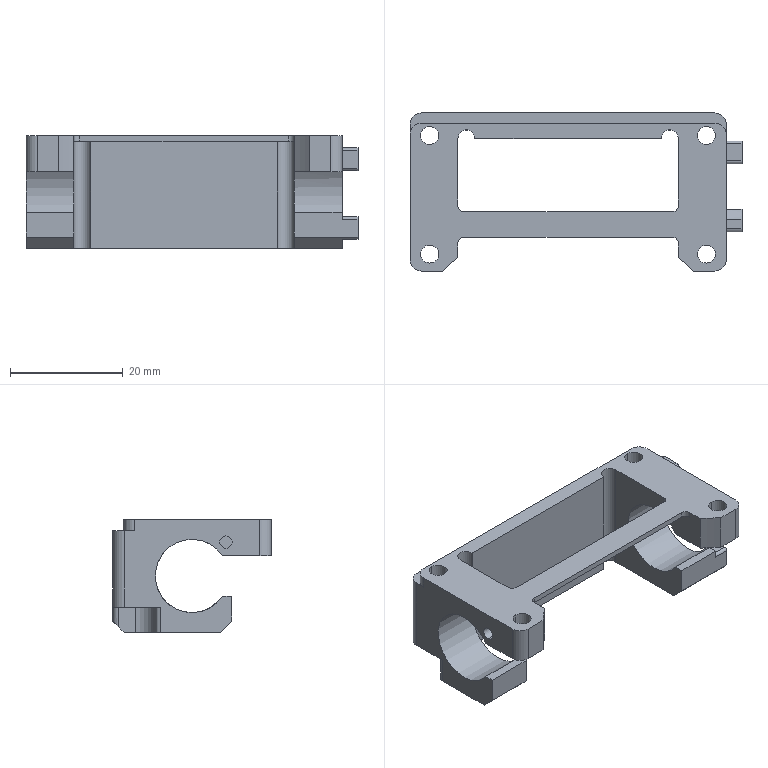NC program | Mastercam | posted with a generic post | part box 58.8 x 28 x 20 mm
Lines 3433 to 4298 of 29451:
(6 FEM |TOOL - 6|DIA. OFF. - 6|LEN. - 6|TOOL DIA. - 6.)
N6930 T6 M6
N6932 G0 G54 G90 X27.5 Y13.92 C0. B0. S6500 M3
N6934 G43 H6 Z50.
N6936 Z.11
N6938 G1 X27.215 Y13.9 Z.1 F2500.
N6940 X26.937 Y13.839 Z.09
N6942 X26.669 Y13.739 Z.08
N6944 X26.419 Y13.603 Z.07
N6946 X26.19 Y13.432 Z.06
N6948 X25.989 Y13.23 Z.05
N6950 X25.817 Y13.001 Z.04
N6952 X25.681 Y12.751 Z.03
N6954 X25.581 Y12.484 Z.02
N6956 X25.52 Y12.205 Z.01
N6958 X25.5 Y11.92 Z0.
N6960 Y10.158
N6962 X25.523 Y9.924
N6964 X25.581 Y9.785
N6966 X25.686 Y9.68
N6968 X25.825 Y9.622
N6970 X27.799 Y9.6
N6972 X28.084 Y9.617 Z.01
N6974 X28.364 Y9.675 Z.02
N6976 X28.632 Y9.771 Z.03
N6978 X28.884 Y9.905 Z.04
N6980 X29.115 Y10.074 Z.05
N6982 X29.319 Y10.273 Z.06
N6984 X29.492 Y10.5 Z.07
N6986 X29.632 Y10.748 Z.08
N6988 X29.735 Y11.015 Z.09
N6990 X29.798 Y11.293 Z.1
N6992 X29.822 Y11.577 Z.11
N6994 X29.823 Y11.655
N6996 X29.825 Y11.731 Z.109
N6998 X29.826 Y11.805
N7000 X29.828 Y11.878 Z.108
N7002 X29.831 Y11.95 Z.107
N7004 X29.833 Y12.02
N7006 X29.836 Y12.088 Z.105
N7008 X29.839 Y12.155 Z.104
N7010 X29.846 Y12.285 Z.101
N7012 X29.853 Y12.408 Z.097
N7014 X29.862 Y12.526 Z.093
N7016 X29.87 Y12.639 Z.088
N7018 X29.88 Y12.746 Z.083
N7020 X29.889 Y12.848 Z.077
N7022 X29.899 Y12.945 Z.07
N7024 X29.909 Y13.037 Z.064
N7026 X29.918 Y13.124 Z.056
N7028 X29.928 Y13.206 Z.048
N7030 X29.937 Y13.284 Z.04
N7032 X29.946 Y13.357 Z.032
N7034 X29.954 Y13.426 Z.023
N7036 X29.962 Y13.49 Z.013
N7038 X29.974 Y13.606 Z-.006
N7040 X29.983 Y13.707 Z-.027
N7042 X29.985 Y13.752 Z-.038
N7044 X29.986 Y13.793 Z-.048
N7046 Y13.831 Z-.06
N7048 X29.984 Y13.865 Z-.071
N7050 X29.98 Y13.897 Z-.082
N7052 X29.974 Y13.925 Z-.094
N7054 X29.966 Y13.95 Z-.105
N7056 X29.956 Y13.973 Z-.117
N7058 X29.944 Y13.993 Z-.129
N7060 X29.93 Y14.01 Z-.14
N7062 X29.913 Y14.025 Z-.152
N7064 X29.894 Y14.037 Z-.164
N7066 X29.871 Y14.048 Z-.175
N7068 X29.846 Y14.056 Z-.187
N7070 X29.818 Y14.062 Z-.198
N7072 X29.787 Y14.067 Z-.21
N7074 X29.753 Y14.069 Z-.221
N7076 X29.715 Y14.07 Z-.232
N7078 X29.674 Z-.243
N7080 X29.629 Y14.068 Z-.254
N7082 X29.529 Y14.061 Z-.274
N7084 X29.413 Y14.05 Z-.294
N7086 X29.348 Y14.043 Z-.303
N7088 X29.28 Y14.036 Z-.312
N7090 X29.207 Y14.028 Z-.321
N7092 X29.129 Y14.02 Z-.329
N7094 X29.047 Y14.012 Z-.337
N7096 X28.96 Y14.003 Z-.344
N7098 X28.868 Y13.994 Z-.351
N7100 X28.771 Y13.986 Z-.357
N7102 X28.669 Y13.978 Z-.363
N7104 X28.562 Y13.97 Z-.369
N7106 X28.449 Y13.962 Z-.374
N7108 X28.331 Y13.955 Z-.378
N7110 X28.207 Y13.949 Z-.382
N7112 X28.078 Y13.944 Z-.385
N7114 X28.011 Y13.942 Z-.386
N7116 X27.942 Y13.94 Z-.387
N7118 X27.873 Y13.938 Z-.388
N7120 X27.801 Y13.936 Z-.389
N7122 X27.728 Y13.935
N7124 X27.654 Y13.934 Z-.39
N7126 X27.578
N7128 X27.5
N7130 X27.215 Y13.913 Z-.4
N7132 X26.936 Y13.853 Z-.41
N7134 X26.669 Y13.753 Z-.42
N7136 X26.419 Y13.616 Z-.43
N7138 X26.19 Y13.445 Z-.44
N7140 X25.988 Y13.243 Z-.45
N7142 X25.817 Y13.015 Z-.46
N7144 X25.681 Y12.765 Z-.47
N7146 X25.581 Y12.497 Z-.48
N7148 X25.52 Y12.218 Z-.49
N7150 X25.5 Y11.934 Z-.5
N7152 Y10.158
N7154 X25.523 Y9.924
N7156 X25.581 Y9.785
N7158 X25.686 Y9.68
N7160 X25.825 Y9.622
N7162 X27.799 Y9.6
N7164 X28.084 Y9.617 Z-.49
N7166 X28.364 Y9.675 Z-.48
N7168 X28.632 Y9.771 Z-.47
N7170 X28.884 Y9.905 Z-.46
N7172 X29.115 Y10.074 Z-.45
N7174 X29.319 Y10.273 Z-.44
N7176 X29.492 Y10.5 Z-.43
N7178 X29.632 Y10.748 Z-.42
N7180 X29.735 Y11.015 Z-.41
N7182 X29.798 Y11.293 Z-.4
N7184 X29.822 Y11.577 Z-.39
N7186 X29.823 Y11.655
N7188 X29.824 Y11.73 Z-.391
N7190 X29.826 Y11.805
N7192 X29.828 Y11.877 Z-.392
N7194 X29.83 Y11.949 Z-.393
N7196 X29.833 Y12.018
N7198 X29.836 Y12.087 Z-.395
N7200 X29.839 Y12.153 Z-.396
N7202 X29.846 Y12.282 Z-.399
N7204 X29.853 Y12.406 Z-.403
N7206 X29.861 Y12.523 Z-.407
N7208 X29.87 Y12.636 Z-.412
N7210 X29.879 Y12.743 Z-.417
N7212 X29.889 Y12.844 Z-.423
N7214 X29.898 Y12.941 Z-.43
N7216 X29.908 Y13.032 Z-.436
N7218 X29.917 Y13.119 Z-.444
N7220 X29.927 Y13.201 Z-.452
N7222 X29.936 Y13.278 Z-.46
N7224 X29.944 Y13.351 Z-.468
N7226 X29.952 Y13.419 Z-.477
N7228 X29.96 Y13.483 Z-.487
N7230 X29.972 Y13.599 Z-.506
N7232 X29.98 Y13.699 Z-.527
N7234 X29.983 Y13.744 Z-.538
N7236 X29.984 Y13.785 Z-.548
N7238 X29.983 Y13.822 Z-.56
N7240 X29.981 Y13.856 Z-.571
N7242 X29.977 Y13.888 Z-.582
N7244 X29.971 Y13.916 Z-.594
N7246 X29.963 Y13.941 Z-.605
N7248 X29.953 Y13.963 Z-.617
N7250 X29.941 Y13.983 Z-.629
N7252 X29.926 Y14. Z-.64
N7254 X29.909 Y14.014 Z-.652
N7256 X29.89 Y14.027 Z-.664
N7258 X29.867 Y14.037 Z-.675
N7260 X29.842 Y14.045 Z-.687
N7262 X29.814 Y14.051 Z-.698
N7264 X29.783 Y14.055 Z-.71
N7266 X29.749 Y14.057 Z-.721
N7268 X29.711 Y14.058 Z-.732
N7270 X29.67 Z-.743
N7272 X29.625 Y14.056 Z-.754
N7274 X29.525 Y14.049 Z-.774
N7276 X29.408 Y14.037 Z-.794
N7278 X29.344 Y14.031 Z-.803
N7280 X29.276 Y14.023 Z-.812
N7282 X29.203 Y14.015 Z-.821
N7284 X29.125 Y14.007 Z-.829
N7286 X29.043 Y13.998 Z-.837
N7288 X28.956 Y13.99 Z-.844
N7290 X28.865 Y13.981 Z-.851
N7292 X28.768 Y13.973 Z-.857
N7294 X28.666 Y13.964 Z-.863
N7296 X28.559 Y13.956 Z-.869
N7298 X28.447 Y13.949 Z-.874
N7300 X28.329 Y13.942 Z-.878
N7302 X28.205 Y13.936 Z-.882
N7304 X28.076 Y13.93 Z-.885
N7306 X28.01 Y13.928 Z-.886
N7308 X27.941 Y13.926 Z-.887
N7310 X27.872 Y13.924 Z-.888
N7312 X27.8 Y13.923 Z-.889
N7314 X27.728 Y13.922
N7316 X27.653 Y13.921 Z-.89
N7318 X27.577 Y13.92
N7320 X27.5
N7322 X27.215 Y13.9 Z-.9
N7324 X26.937 Y13.839 Z-.91
N7326 X26.669 Y13.739 Z-.92
N7328 X26.419 Y13.603 Z-.93
N7330 X26.19 Y13.432 Z-.94
N7332 X25.989 Y13.23 Z-.95
N7334 X25.817 Y13.001 Z-.96
N7336 X25.681 Y12.751 Z-.97
N7338 X25.581 Y12.484 Z-.98
N7340 X25.52 Y12.205 Z-.99
N7342 X25.5 Y11.92 Z-1.
N7344 Y10.158
N7346 X25.523 Y9.924
N7348 X25.581 Y9.785
N7350 X25.686 Y9.68
N7352 X25.825 Y9.622
N7354 X27.799 Y9.6
N7356 X28.084 Y9.617 Z-.99
N7358 X28.364 Y9.675 Z-.98
N7360 X28.632 Y9.771 Z-.97
N7362 X28.884 Y9.905 Z-.96
N7364 X29.115 Y10.074 Z-.95
N7366 X29.319 Y10.273 Z-.94
N7368 X29.492 Y10.5 Z-.93
N7370 X29.632 Y10.748 Z-.92
N7372 X29.735 Y11.015 Z-.91
N7374 X29.798 Y11.293 Z-.9
N7376 X29.822 Y11.577 Z-.89
N7378 X29.823 Y11.655
N7380 X29.824 Y11.73 Z-.891
N7382 X29.826 Y11.805
N7384 X29.828 Y11.877 Z-.892
N7386 X29.83 Y11.949 Z-.893
N7388 X29.833 Y12.018
N7390 X29.836 Y12.086 Z-.895
N7392 X29.839 Y12.153 Z-.896
N7394 X29.846 Y12.282 Z-.899
N7396 X29.853 Y12.406 Z-.903
N7398 X29.861 Y12.523 Z-.907
N7400 X29.87 Y12.635 Z-.912
N7402 X29.879 Y12.742 Z-.917
N7404 X29.888 Y12.844 Z-.923
N7406 X29.898 Y12.94 Z-.929
N7408 X29.908 Y13.032 Z-.936
N7410 X29.917 Y13.119 Z-.943
N7412 X29.927 Y13.2 Z-.951
N7414 X29.936 Y13.278 Z-.959
N7416 X29.944 Y13.35 Z-.968
N7418 X29.952 Y13.419 Z-.977
N7420 X29.96 Y13.483 Z-.986
N7422 X29.972 Y13.599 Z-1.005
N7424 X29.98 Y13.699 Z-1.026
N7426 X29.983 Y13.743 Z-1.036
N7428 Y13.784 Z-1.047
N7430 Y13.822 Z-1.058
N7432 X29.981 Y13.856 Z-1.069
N7434 X29.977 Y13.887 Z-1.08
N7436 X29.971 Y13.915 Z-1.092
N7438 X29.963 Y13.94 Z-1.103
N7440 X29.953 Y13.963 Z-1.115
N7442 X29.941 Y13.982 Z-1.126
N7444 X29.926 Y13.999 Z-1.138
N7446 X29.909 Y14.014 Z-1.15
N7448 X29.889 Y14.026 Z-1.161
N7450 X29.867 Y14.036 Z-1.173
N7452 X29.842 Y14.044 Z-1.184
N7454 X29.814 Y14.051 Z-1.195
N7456 X29.783 Y14.055 Z-1.207
N7458 X29.748 Y14.057 Z-1.218
N7460 X29.711 Y14.058 Z-1.229
N7462 X29.669 Z-1.24
N7464 X29.625 Y14.056 Z-1.25
N7466 X29.524 Y14.048 Z-1.271
N7468 X29.408 Y14.037 Z-1.29
N7470 X29.344 Y14.03 Z-1.299
N7472 X29.275 Y14.023 Z-1.308
N7474 X29.202 Y14.015 Z-1.317
N7476 X29.125 Y14.007 Z-1.325
N7478 X29.043 Y13.998 Z-1.333
N7480 X28.956 Y13.99 Z-1.34
N7482 X28.864 Y13.981 Z-1.347
N7484 X28.768 Y13.972 Z-1.353
N7486 X28.666 Y13.964 Z-1.359
N7488 X28.559 Y13.956 Z-1.364
N7490 X28.447 Y13.949 Z-1.369
N7492 X28.329 Y13.942 Z-1.373
N7494 X28.205 Y13.936 Z-1.377
N7496 X28.076 Y13.93 Z-1.38
N7498 X28.009 Y13.928 Z-1.381
N7500 X27.941 Y13.926 Z-1.382
N7502 X27.871 Y13.924 Z-1.383
N7504 X27.8 Y13.923 Z-1.384
N7506 X27.727 Y13.922 Z-1.385
N7508 X27.653 Y13.921
N7510 X27.577 Y13.92
N7512 X27.5 Z-1.386
N7514 X27.215 Y13.9 Z-1.396
N7516 X26.937 Y13.839 Z-1.406
N7518 X26.669 Y13.739 Z-1.415
N7520 X26.419 Y13.603 Z-1.425
N7522 X26.19 Y13.432 Z-1.435
N7524 X25.989 Y13.23 Z-1.445
N7526 X25.817 Y13.001 Z-1.455
N7528 X25.681 Y12.751 Z-1.465
N7530 X25.581 Y12.484 Z-1.475
N7532 X25.52 Y12.205 Z-1.485
N7534 X25.5 Y11.92 Z-1.495
N7536 Y10.158
N7538 X25.523 Y9.924
N7540 X25.581 Y9.785
N7542 X25.686 Y9.68
N7544 X25.825 Y9.622
N7546 X27.799 Y9.6
N7548 X28.084 Y9.617 Z-1.485
N7550 X28.364 Y9.675 Z-1.475
N7552 X28.632 Y9.771 Z-1.465
N7554 X28.884 Y9.905 Z-1.455
N7556 X29.115 Y10.074 Z-1.445
N7558 X29.319 Y10.273 Z-1.435
N7560 X29.492 Y10.5 Z-1.425
N7562 X29.632 Y10.748 Z-1.415
N7564 X29.735 Y11.015 Z-1.406
N7566 X29.798 Y11.293 Z-1.396
N7568 X29.822 Y11.577 Z-1.386
N7570 X29.823 Y11.654
N7572 X29.824 Y11.729
N7574 X29.826 Y11.803
N7576 X29.828 Y11.875
N7578 X29.83 Y11.946 Z-1.387
N7580 X29.833 Y12.015
N7582 X29.836 Y12.082 Z-1.388
N7584 X29.838 Y12.149
N7586 X29.845 Y12.277 Z-1.39
N7588 X29.852 Y12.399 Z-1.392
N7590 X29.86 Y12.516 Z-1.394
N7592 X29.869 Y12.628 Z-1.396
N7594 X29.878 Y12.734 Z-1.399
N7596 X29.887 Y12.835 Z-1.402
N7598 X29.896 Y12.931 Z-1.405
N7600 X29.905 Y13.022 Z-1.408
N7602 X29.914 Y13.108 Z-1.412
N7604 X29.923 Y13.189 Z-1.416
N7606 X29.932 Y13.266 Z-1.42
N7608 X29.94 Y13.339 Z-1.424
N7610 X29.948 Y13.407 Z-1.429
N7612 X29.955 Y13.471 Z-1.433
N7614 X29.966 Y13.586 Z-1.443
N7616 X29.974 Y13.686 Z-1.453
N7618 X29.976 Y13.731 Z-1.458
N7620 Y13.772 Z-1.464
N7622 X29.975 Y13.81 Z-1.469
N7624 X29.972 Y13.844 Z-1.475
N7626 X29.968 Y13.875 Z-1.481
N7628 X29.962 Y13.904 Z-1.486
N7630 X29.953 Y13.929 Z-1.492
N7632 X29.943 Y13.952 Z-1.498
N7634 X29.93 Y13.972 Z-1.504
N7636 X29.916 Y13.989 Z-1.509
N7638 X29.898 Y14.004 Z-1.515
N7640 X29.878 Y14.017 Z-1.521
N7642 X29.856 Y14.027 Z-1.527
N7644 X29.83 Y14.036 Z-1.532
N7646 X29.802 Y14.042 Z-1.538
N7648 X29.771 Y14.047 Z-1.544
N7650 X29.736 Y14.05 Z-1.549
N7652 X29.698 Y14.051 Z-1.555
N7654 X29.657 Z-1.56
N7656 X29.612 Y14.049 Z-1.565
N7658 X29.512 Y14.043 Z-1.576
N7660 X29.396 Y14.033 Z-1.585
N7662 X29.332 Y14.026 Z-1.59
N7664 X29.264 Y14.019 Z-1.594
N7666 X29.191 Y14.012 Z-1.599
N7668 X29.114 Y14.004 Z-1.603
N7670 X29.032 Y13.996 Z-1.607
N7672 X28.946 Y13.987 Z-1.61
N7674 X28.855 Y13.979 Z-1.614
N7676 X28.759 Y13.971 Z-1.617
N7678 X28.657 Y13.963 Z-1.62
N7680 X28.551 Y13.955 Z-1.622
N7682 X28.439 Y13.948 Z-1.625
N7684 X28.322 Y13.941 Z-1.627
N7686 X28.2 Y13.935 Z-1.629
N7688 X28.072 Y13.93 Z-1.63
N7690 X28.005 Y13.928 Z-1.631
N7692 X27.938 Y13.926
N7694 X27.868 Y13.924 Z-1.632
N7696 X27.798 Y13.923
N7698 X27.726 Y13.922 Z-1.633
N7700 X27.652 Y13.921
N7702 X27.577 Y13.92
N7704 X27.5
N7706 X27.215 Y13.9 Z-1.643
N7708 X26.937 Y13.839 Z-1.653
N7710 X26.669 Y13.739 Z-1.663
N7712 X26.419 Y13.603 Z-1.673
N7714 X26.19 Y13.432 Z-1.683
N7716 X25.989 Y13.23 Z-1.693
N7718 X25.817 Y13.001 Z-1.703
N7720 X25.681 Y12.751 Z-1.713
N7722 X25.581 Y12.484 Z-1.723
N7724 X25.52 Y12.205 Z-1.733
N7726 X25.5 Y11.92 Z-1.743
N7728 Y10.158
N7730 X25.523 Y9.924
N7732 X25.581 Y9.785
N7734 X25.686 Y9.68
N7736 X25.825 Y9.622
N7738 X27.799 Y9.6
N7740 X28.084 Y9.617 Z-1.733
N7742 X28.364 Y9.675 Z-1.723
N7744 X28.632 Y9.771 Z-1.713
N7746 X28.884 Y9.905 Z-1.703
N7748 X29.115 Y10.074 Z-1.693
N7750 X29.319 Y10.273 Z-1.683
N7752 X29.492 Y10.5 Z-1.673
N7754 X29.632 Y10.748 Z-1.663
N7756 X29.735 Y11.015 Z-1.653
N7758 X29.798 Y11.293 Z-1.643
N7760 X29.822 Y11.577 Z-1.633
N7762 X29.823 Y11.654
N7764 X29.824 Y11.729
N7766 X29.826 Y11.803
N7768 X29.828 Y11.875 Z-1.634
N7770 X29.83 Y11.946
N7772 X29.833 Y12.015 Z-1.635
N7774 X29.836 Y12.082
N7776 X29.839 Y12.149 Z-1.636
N7778 X29.845 Y12.277 Z-1.638
N7780 X29.852 Y12.399 Z-1.639
N7782 X29.86 Y12.516 Z-1.642
N7784 X29.869 Y12.628 Z-1.644
N7786 X29.878 Y12.734 Z-1.647
N7788 X29.887 Y12.835 Z-1.65
N7790 X29.896 Y12.931 Z-1.653
N7792 X29.905 Y13.022 Z-1.657
N7794 X29.914 Y13.108 Z-1.661
N7796 X29.923 Y13.19 Z-1.665
N7798 X29.932 Y13.267 Z-1.669
N7800 X29.94 Y13.339 Z-1.673
N7802 X29.948 Y13.407 Z-1.678
N7804 X29.955 Y13.471 Z-1.683
N7806 X29.967 Y13.587 Z-1.693
N7808 X29.974 Y13.687 Z-1.703
N7810 X29.976 Y13.731 Z-1.709
N7812 Y13.772 Z-1.714
N7814 X29.975 Y13.81 Z-1.72
N7816 X29.973 Y13.845 Z-1.726
N7818 X29.968 Y13.876 Z-1.732
N7820 X29.962 Y13.904 Z-1.738
N7822 X29.954 Y13.929 Z-1.744
N7824 X29.943 Y13.952 Z-1.75
N7826 X29.931 Y13.972 Z-1.756
N7828 X29.916 Y13.989 Z-1.762
N7830 X29.899 Y14.004 Z-1.768
N7832 X29.879 Y14.017 Z-1.774
N7834 X29.856 Y14.027 Z-1.78
N7836 X29.831 Y14.036 Z-1.786
N7838 X29.802 Y14.042 Z-1.792
N7840 X29.771 Y14.047 Z-1.797
N7842 X29.736 Y14.05 Z-1.803
N7844 X29.699 Y14.051 Z-1.809
N7846 X29.657 Z-1.815
N7848 X29.613 Y14.05 Z-1.82
N7850 X29.512 Y14.043 Z-1.831
N7852 X29.396 Y14.033 Z-1.841
N7854 X29.332 Y14.026 Z-1.845
N7856 X29.264 Y14.019 Z-1.85
N7858 X29.191 Y14.012 Z-1.855
N7860 X29.114 Y14.004 Z-1.859
N7862 X29.033 Y13.996 Z-1.863
N7864 X28.946 Y13.987 Z-1.867
N7866 X28.855 Y13.979 Z-1.87
N7868 X28.759 Y13.971 Z-1.873
N7870 X28.658 Y13.963 Z-1.876
N7872 X28.551 Y13.955 Z-1.879
N7874 X28.44 Y13.948 Z-1.882
N7876 X28.323 Y13.941 Z-1.884
N7878 X28.2 Y13.935 Z-1.886
N7880 X28.072 Y13.93 Z-1.887
N7882 X28.005 Y13.928 Z-1.888
N7884 X27.938 Y13.926 Z-1.889
N7886 X27.869 Y13.924
N7888 X27.798 Y13.923 Z-1.89
N7890 X27.726 Y13.922
N7892 X27.652 Y13.921
N7894 X27.577 Y13.92
N7896 X27.5
N7898 X27.215 Y13.9 Z-1.9
N7900 X26.937 Y13.839 Z-1.91
N7902 X26.669 Y13.739 Z-1.92
N7904 X26.419 Y13.603 Z-1.93
N7906 X26.19 Y13.432 Z-1.94
N7908 X25.989 Y13.23 Z-1.95
N7910 X25.817 Y13.001 Z-1.96
N7912 X25.681 Y12.751 Z-1.97
N7914 X25.581 Y12.484 Z-1.98
N7916 X25.52 Y12.205 Z-1.99
N7918 X25.5 Y11.92 Z-2.
N7920 Y10.158
N7922 X25.523 Y9.924
N7924 X25.581 Y9.785
N7926 X25.686 Y9.68
N7928 X25.825 Y9.622
N7930 X27.799 Y9.6
N7932 X28.084 Y9.617 Z-1.99
N7934 X28.364 Y9.675 Z-1.98
N7936 X28.632 Y9.771 Z-1.97
N7938 X28.884 Y9.905 Z-1.96
N7940 X29.115 Y10.074 Z-1.95
N7942 X29.319 Y10.273 Z-1.94
N7944 X29.492 Y10.5 Z-1.93
N7946 X29.632 Y10.748 Z-1.92
N7948 X29.735 Y11.015 Z-1.91
N7950 X29.798 Y11.293 Z-1.9
N7952 X29.822 Y11.577 Z-1.89
N7954 X29.823 Y11.655
N7956 X29.824 Y11.73 Z-1.891
N7958 X29.826 Y11.805
N7960 X29.828 Y11.877 Z-1.892
N7962 X29.83 Y11.949 Z-1.893
N7964 X29.833 Y12.018
N7966 X29.836 Y12.087 Z-1.895
N7968 X29.839 Y12.153 Z-1.896
N7970 X29.846 Y12.282 Z-1.899
N7972 X29.853 Y12.406 Z-1.903
N7974 X29.861 Y12.523 Z-1.907
N7976 X29.87 Y12.636 Z-1.912
N7978 X29.879 Y12.743 Z-1.917
N7980 X29.889 Y12.844 Z-1.923
N7982 X29.898 Y12.941 Z-1.93
N7984 X29.908 Y13.032 Z-1.936
N7986 X29.917 Y13.119 Z-1.944
N7988 X29.927 Y13.201 Z-1.952
N7990 X29.936 Y13.278 Z-1.96
N7992 X29.944 Y13.351 Z-1.968
N7994 X29.952 Y13.419 Z-1.977
N7996 X29.96 Y13.483 Z-1.987
N7998 X29.972 Y13.599 Z-2.006
N8000 X29.98 Y13.699 Z-2.027
N8002 X29.983 Y13.744 Z-2.038
N8004 X29.984 Y13.785 Z-2.048
N8006 X29.983 Y13.822 Z-2.06
N8008 X29.981 Y13.856 Z-2.071
N8010 X29.977 Y13.888 Z-2.082
N8012 X29.971 Y13.916 Z-2.094
N8014 X29.963 Y13.941 Z-2.105
N8016 X29.953 Y13.963 Z-2.117
N8018 X29.941 Y13.983 Z-2.129
N8020 X29.926 Y14. Z-2.14
N8022 X29.909 Y14.014 Z-2.152
N8024 X29.89 Y14.027 Z-2.164
N8026 X29.867 Y14.037 Z-2.175
N8028 X29.842 Y14.045 Z-2.187
N8030 X29.814 Y14.051 Z-2.198
N8032 X29.783 Y14.055 Z-2.21
N8034 X29.749 Y14.057 Z-2.221
N8036 X29.711 Y14.058 Z-2.232
N8038 X29.67 Z-2.243
N8040 X29.625 Y14.056 Z-2.254
N8042 X29.525 Y14.049 Z-2.274
N8044 X29.408 Y14.037 Z-2.294
N8046 X29.344 Y14.031 Z-2.303
N8048 X29.276 Y14.023 Z-2.312
N8050 X29.203 Y14.015 Z-2.321
N8052 X29.125 Y14.007 Z-2.329
N8054 X29.043 Y13.998 Z-2.337
N8056 X28.956 Y13.99 Z-2.344
N8058 X28.865 Y13.981 Z-2.351
N8060 X28.768 Y13.973 Z-2.357
N8062 X28.666 Y13.964 Z-2.363
N8064 X28.559 Y13.956 Z-2.369
N8066 X28.447 Y13.949 Z-2.374
N8068 X28.329 Y13.942 Z-2.378
N8070 X28.205 Y13.936 Z-2.382
N8072 X28.076 Y13.93 Z-2.385
N8074 X28.01 Y13.928 Z-2.386
N8076 X27.941 Y13.926 Z-2.387
N8078 X27.872 Y13.924 Z-2.388
N8080 X27.8 Y13.923 Z-2.389
N8082 X27.728 Y13.922
N8084 X27.653 Y13.921 Z-2.39
N8086 X27.577 Y13.92
N8088 X27.5
N8090 X27.215 Y13.9 Z-2.4
N8092 X26.937 Y13.839 Z-2.41
N8094 X26.669 Y13.739 Z-2.42
N8096 X26.419 Y13.603 Z-2.43
N8098 X26.19 Y13.432 Z-2.44
N8100 X25.989 Y13.23 Z-2.45
N8102 X25.817 Y13.001 Z-2.46
N8104 X25.681 Y12.751 Z-2.47
N8106 X25.581 Y12.484 Z-2.48
N8108 X25.52 Y12.205 Z-2.49
N8110 X25.5 Y11.92 Z-2.5
N8112 Y10.158
N8114 X25.523 Y9.924
N8116 X25.581 Y9.785
N8118 X25.686 Y9.68
N8120 X25.825 Y9.622
N8122 X27.799 Y9.6
N8124 X28.084 Y9.617 Z-2.49
N8126 X28.364 Y9.675 Z-2.48
N8128 X28.632 Y9.771 Z-2.47
N8130 X28.884 Y9.905 Z-2.46
N8132 X29.115 Y10.074 Z-2.45
N8134 X29.319 Y10.273 Z-2.44
N8136 X29.492 Y10.5 Z-2.43
N8138 X29.632 Y10.748 Z-2.42
N8140 X29.735 Y11.015 Z-2.41
N8142 X29.798 Y11.293 Z-2.4
N8144 X29.822 Y11.577 Z-2.39
N8146 X29.823 Y11.655
N8148 X29.824 Y11.73 Z-2.391
N8150 X29.826 Y11.805
N8152 X29.828 Y11.877 Z-2.392
N8154 X29.83 Y11.949 Z-2.393
N8156 X29.833 Y12.018
N8158 X29.836 Y12.087 Z-2.395
N8160 X29.839 Y12.153 Z-2.396
N8162 X29.846 Y12.282 Z-2.399
N8164 X29.853 Y12.406 Z-2.403
N8166 X29.861 Y12.523 Z-2.407
N8168 X29.87 Y12.636 Z-2.412
N8170 X29.879 Y12.743 Z-2.417
N8172 X29.889 Y12.844 Z-2.423
N8174 X29.898 Y12.941 Z-2.43
N8176 X29.908 Y13.032 Z-2.436
N8178 X29.917 Y13.119 Z-2.444
N8180 X29.927 Y13.201 Z-2.452
N8182 X29.936 Y13.278 Z-2.46
N8184 X29.944 Y13.351 Z-2.468
N8186 X29.952 Y13.419 Z-2.477
N8188 X29.96 Y13.483 Z-2.487
N8190 X29.972 Y13.599 Z-2.506
N8192 X29.98 Y13.699 Z-2.527
N8194 X29.983 Y13.744 Z-2.538
N8196 X29.984 Y13.785 Z-2.548
N8198 X29.983 Y13.822 Z-2.56
N8200 X29.981 Y13.856 Z-2.571
N8202 X29.977 Y13.888 Z-2.582
N8204 X29.971 Y13.916 Z-2.594
N8206 X29.963 Y13.941 Z-2.605
N8208 X29.953 Y13.963 Z-2.617
N8210 X29.941 Y13.983 Z-2.629
N8212 X29.926 Y14. Z-2.64
N8214 X29.909 Y14.014 Z-2.652
N8216 X29.89 Y14.027 Z-2.664
N8218 X29.867 Y14.037 Z-2.675
N8220 X29.842 Y14.045 Z-2.687
N8222 X29.814 Y14.051 Z-2.698
N8224 X29.783 Y14.055 Z-2.71
N8226 X29.749 Y14.057 Z-2.721
N8228 X29.711 Y14.058 Z-2.732
N8230 X29.67 Z-2.743
N8232 X29.625 Y14.056 Z-2.754
N8234 X29.525 Y14.049 Z-2.774
N8236 X29.408 Y14.037 Z-2.794
N8238 X29.344 Y14.031 Z-2.803
N8240 X29.276 Y14.023 Z-2.812
N8242 X29.203 Y14.015 Z-2.821
N8244 X29.125 Y14.007 Z-2.829
N8246 X29.043 Y13.998 Z-2.837
N8248 X28.956 Y13.99 Z-2.844
N8250 X28.865 Y13.981 Z-2.851
N8252 X28.768 Y13.973 Z-2.857
N8254 X28.666 Y13.964 Z-2.863
N8256 X28.559 Y13.956 Z-2.869
N8258 X28.447 Y13.949 Z-2.874
N8260 X28.329 Y13.942 Z-2.878
N8262 X28.205 Y13.936 Z-2.882
N8264 X28.076 Y13.93 Z-2.885
N8266 X28.01 Y13.928 Z-2.886
N8268 X27.941 Y13.926 Z-2.887
N8270 X27.872 Y13.924 Z-2.888
N8272 X27.8 Y13.923 Z-2.889
N8274 X27.728 Y13.922
N8276 X27.653 Y13.921 Z-2.89
N8278 X27.577 Y13.92
N8280 X27.5
N8282 X27.215 Y13.9 Z-2.9
N8284 X26.937 Y13.839 Z-2.91
N8286 X26.669 Y13.739 Z-2.92
N8288 X26.419 Y13.603 Z-2.93
N8290 X26.19 Y13.432 Z-2.94
N8292 X25.989 Y13.23 Z-2.95
N8294 X25.817 Y13.001 Z-2.96
N8296 X25.681 Y12.751 Z-2.97
N8298 X25.581 Y12.484 Z-2.98
N8300 X25.52 Y12.205 Z-2.99
N8302 X25.5 Y11.92 Z-3.
N8304 Y10.158
N8306 X25.523 Y9.924
N8308 X25.581 Y9.785
N8310 X25.686 Y9.68
N8312 X25.825 Y9.622
N8314 X27.799 Y9.6
N8316 X28.084 Y9.617 Z-2.99
N8318 X28.364 Y9.675 Z-2.98
N8320 X28.632 Y9.771 Z-2.97
N8322 X28.884 Y9.905 Z-2.96
N8324 X29.115 Y10.074 Z-2.95
N8326 X29.319 Y10.273 Z-2.94
N8328 X29.492 Y10.5 Z-2.93
N8330 X29.632 Y10.748 Z-2.92
N8332 X29.735 Y11.015 Z-2.91
N8334 X29.798 Y11.293 Z-2.9
N8336 X29.822 Y11.577 Z-2.89
N8338 X29.823 Y11.655
N8340 X29.824 Y11.73 Z-2.891
N8342 X29.826 Y11.805
N8344 X29.828 Y11.877 Z-2.892
N8346 X29.83 Y11.949 Z-2.893
N8348 X29.833 Y12.018
N8350 X29.836 Y12.087 Z-2.895
N8352 X29.839 Y12.153 Z-2.896
N8354 X29.846 Y12.282 Z-2.899
N8356 X29.853 Y12.406 Z-2.903
N8358 X29.861 Y12.523 Z-2.907
N8360 X29.87 Y12.636 Z-2.912
N8362 X29.879 Y12.743 Z-2.917
N8364 X29.889 Y12.844 Z-2.923
N8366 X29.898 Y12.941 Z-2.93
N8368 X29.908 Y13.032 Z-2.936
N8370 X29.917 Y13.119 Z-2.944
N8372 X29.927 Y13.201 Z-2.952
N8374 X29.936 Y13.278 Z-2.96
N8376 X29.944 Y13.351 Z-2.968
N8378 X29.952 Y13.419 Z-2.977
N8380 X29.96 Y13.483 Z-2.987
N8382 X29.972 Y13.599 Z-3.006
N8384 X29.98 Y13.699 Z-3.027
N8386 X29.983 Y13.744 Z-3.038
N8388 X29.984 Y13.785 Z-3.048
N8390 X29.983 Y13.822 Z-3.06
N8392 X29.981 Y13.856 Z-3.071
N8394 X29.977 Y13.888 Z-3.082
N8396 X29.971 Y13.916 Z-3.094
N8398 X29.963 Y13.941 Z-3.105
N8400 X29.953 Y13.963 Z-3.117
N8402 X29.941 Y13.983 Z-3.129
N8404 X29.926 Y14. Z-3.14
N8406 X29.909 Y14.014 Z-3.152
N8408 X29.89 Y14.027 Z-3.164
N8410 X29.867 Y14.037 Z-3.175
N8412 X29.842 Y14.045 Z-3.187
N8414 X29.814 Y14.051 Z-3.198
N8416 X29.783 Y14.055 Z-3.21
N8418 X29.749 Y14.057 Z-3.221
N8420 X29.711 Y14.058 Z-3.232
N8422 X29.67 Z-3.243
N8424 X29.625 Y14.056 Z-3.254
N8426 X29.525 Y14.049 Z-3.274
N8428 X29.408 Y14.037 Z-3.294
N8430 X29.344 Y14.031 Z-3.303
N8432 X29.276 Y14.023 Z-3.312
N8434 X29.203 Y14.015 Z-3.321
N8436 X29.125 Y14.007 Z-3.329
N8438 X29.043 Y13.998 Z-3.337
N8440 X28.956 Y13.99 Z-3.344
N8442 X28.865 Y13.981 Z-3.351
N8444 X28.768 Y13.973 Z-3.357
N8446 X28.666 Y13.964 Z-3.363
N8448 X28.559 Y13.956 Z-3.369
N8450 X28.447 Y13.949 Z-3.374
N8452 X28.329 Y13.942 Z-3.378
N8454 X28.205 Y13.936 Z-3.382
N8456 X28.076 Y13.93 Z-3.385
N8458 X28.01 Y13.928 Z-3.386
N8460 X27.941 Y13.926 Z-3.387
N8462 X27.872 Y13.924 Z-3.388
N8464 X27.8 Y13.923 Z-3.389
N8466 X27.728 Y13.922
N8468 X27.653 Y13.921 Z-3.39
N8470 X27.577 Y13.92
N8472 X27.5
N8474 X27.215 Y13.9 Z-3.4
N8476 X26.937 Y13.839 Z-3.41
N8478 X26.669 Y13.739 Z-3.42
N8480 X26.419 Y13.603 Z-3.43
N8482 X26.19 Y13.432 Z-3.44
N8484 X25.989 Y13.23 Z-3.45
N8486 X25.817 Y13.001 Z-3.46
N8488 X25.681 Y12.751 Z-3.47
N8490 X25.581 Y12.484 Z-3.48
N8492 X25.52 Y12.205 Z-3.49
N8494 X25.5 Y11.92 Z-3.5
N8496 Y10.158
N8498 X25.523 Y9.924
N8500 X25.581 Y9.785
N8502 X25.686 Y9.68
N8504 X25.825 Y9.622
N8506 X27.799 Y9.6
N8508 X28.084 Y9.617 Z-3.49
N8510 X28.364 Y9.675 Z-3.48
N8512 X28.632 Y9.771 Z-3.47
N8514 X28.884 Y9.905 Z-3.46
N8516 X29.115 Y10.074 Z-3.45
N8518 X29.319 Y10.273 Z-3.44
N8520 X29.492 Y10.5 Z-3.43
N8522 X29.632 Y10.748 Z-3.42
N8524 X29.735 Y11.015 Z-3.41
N8526 X29.798 Y11.293 Z-3.4
N8528 X29.822 Y11.577 Z-3.39
N8530 X29.823 Y11.655
N8532 X29.824 Y11.73 Z-3.391
N8534 X29.826 Y11.805
N8536 X29.828 Y11.877 Z-3.392
N8538 X29.83 Y11.949 Z-3.393
N8540 X29.833 Y12.018
N8542 X29.836 Y12.087 Z-3.395
N8544 X29.839 Y12.153 Z-3.396
N8546 X29.846 Y12.282 Z-3.399
N8548 X29.853 Y12.406 Z-3.403
N8550 X29.861 Y12.523 Z-3.407
N8552 X29.87 Y12.636 Z-3.412
N8554 X29.879 Y12.743 Z-3.417
N8556 X29.889 Y12.844 Z-3.423
N8558 X29.898 Y12.941 Z-3.43
N8560 X29.908 Y13.032 Z-3.436
N8562 X29.917 Y13.119 Z-3.444
N8564 X29.927 Y13.201 Z-3.452
N8566 X29.936 Y13.278 Z-3.46
N8568 X29.944 Y13.351 Z-3.468
N8570 X29.952 Y13.419 Z-3.477
N8572 X29.96 Y13.483 Z-3.487
N8574 X29.972 Y13.599 Z-3.506
N8576 X29.98 Y13.699 Z-3.527
N8578 X29.983 Y13.744 Z-3.538
N8580 X29.984 Y13.785 Z-3.548
N8582 X29.983 Y13.822 Z-3.56
N8584 X29.981 Y13.856 Z-3.571
N8586 X29.977 Y13.888 Z-3.582
N8588 X29.971 Y13.916 Z-3.594
N8590 X29.963 Y13.941 Z-3.605
N8592 X29.953 Y13.963 Z-3.617
N8594 X29.941 Y13.983 Z-3.629
N8596 X29.926 Y14. Z-3.64
N8598 X29.909 Y14.014 Z-3.652
N8600 X29.89 Y14.027 Z-3.664
N8602 X29.867 Y14.037 Z-3.675
N8604 X29.842 Y14.045 Z-3.687
N8606 X29.814 Y14.051 Z-3.698
N8608 X29.783 Y14.055 Z-3.71
N8610 X29.749 Y14.057 Z-3.721
N8612 X29.711 Y14.058 Z-3.732
N8614 X29.67 Z-3.743
N8616 X29.625 Y14.056 Z-3.754
N8618 X29.525 Y14.049 Z-3.774
N8620 X29.408 Y14.037 Z-3.794
N8622 X29.344 Y14.031 Z-3.803
N8624 X29.276 Y14.023 Z-3.812
N8626 X29.203 Y14.015 Z-3.821
N8628 X29.125 Y14.007 Z-3.829
N8630 X29.043 Y13.998 Z-3.837
N8632 X28.956 Y13.99 Z-3.844
N8634 X28.865 Y13.981 Z-3.851
N8636 X28.768 Y13.973 Z-3.857
N8638 X28.666 Y13.964 Z-3.863
N8640 X28.559 Y13.956 Z-3.869
N8642 X28.447 Y13.949 Z-3.874
N8644 X28.329 Y13.942 Z-3.878
N8646 X28.205 Y13.936 Z-3.882
N8648 X28.076 Y13.93 Z-3.885
N8650 X28.01 Y13.928 Z-3.886
N8652 X27.941 Y13.926 Z-3.887
N8654 X27.872 Y13.924 Z-3.888
N8656 X27.8 Y13.923 Z-3.889
N8658 X27.728 Y13.922